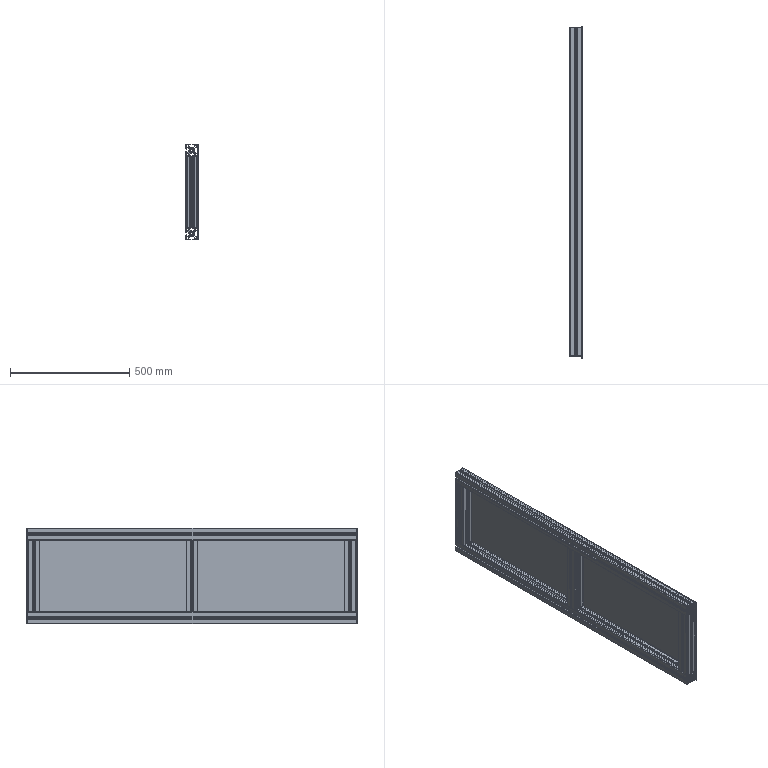Part | SolidWorks | features ICE 1, WeldMemberFeat 1, WeldmentFeature 1 | 6 solids | 1265 faces | box 51.5 x 1389 x 400 mm | volume 4308488 mm3 | cylinder 729 | plane 536 | commonest cylinder face diameters 0.4 x200 0.8 x200 2 x90 10 x60 1 x50 10.2 x45